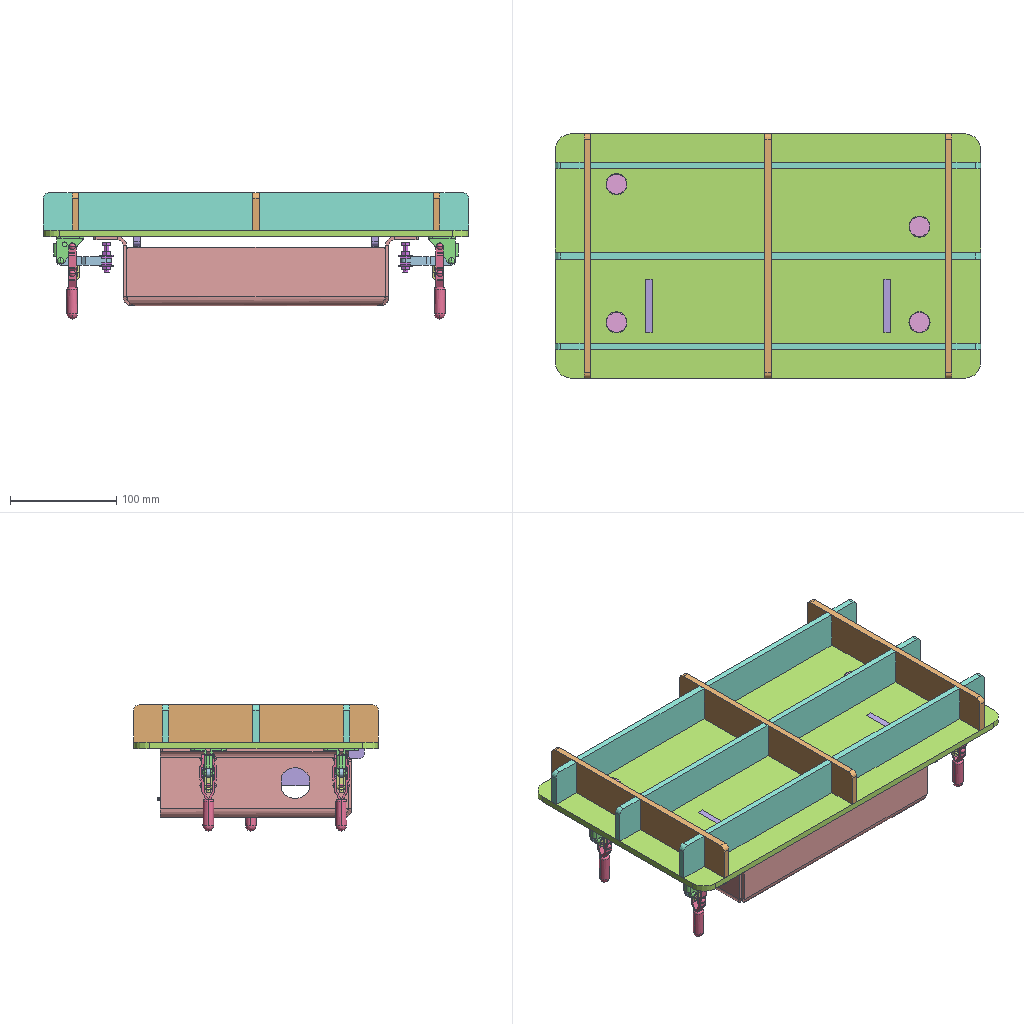Assembly | SolidWorks | 8 different items | 20 placed | box 400 x 230 x 119 mm
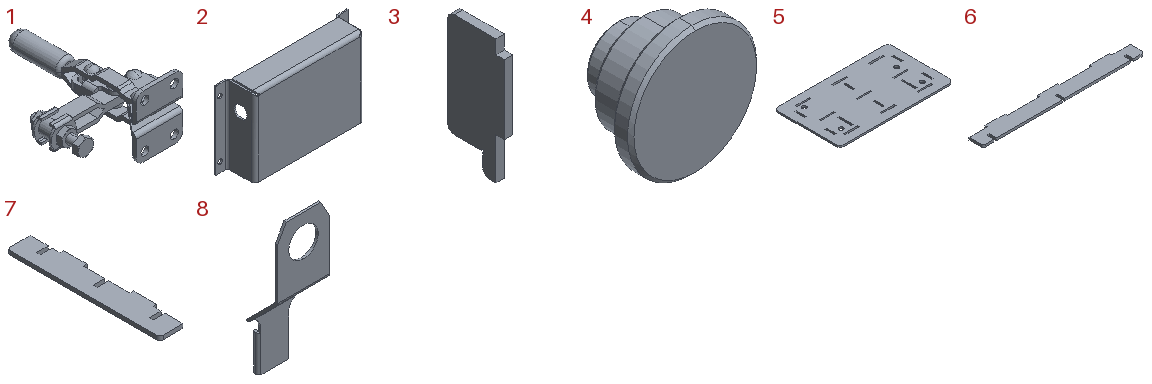Parts list (item | quantity | size | volume | features):
1 | x4 | 56.45 x 77.62 x 33.3 mm | 10418 mm3 | features BaseBody 5
2 | x1 | 305 x 65 x 180.2 mm | 266620 mm3 | features ICE 3, EdgeFlange 2, Fillet 1, FlatPattern 1, Fold 1, SMBaseFlange 1, SheetMetal 1, UnFold 1
3 | x2 | 6 x 41 x 90 mm | 18294 mm3 | features FlatPattern 1, SMBaseFlange 1, SheetMetal 1
4 | x4 | 20 x 12.2 x 20 mm | 2180 mm3 | features Chamfer 1, Revolution 1
5 | x1 | 400 x 230 x 6 mm | 519240 mm3 | features FlatPattern 1, SMBaseFlange 1, SheetMetal 1
6 | x3 | 400 x 40.5 x 6 mm | 86942 mm3 | features FlatPattern 1, SMBaseFlange 1, SheetMetal 1
7 | x3 | 40.5 x 230 x 6 mm | 48656 mm3 | features FlatPattern 1, SMBaseFlange 1, SheetMetal 1
8 | x2 | 23.06 x 15.573 x 65.7 mm | 1342 mm3 | features BaseBody 1
Mates (type | each side: item.copy, entity, surface, feature):
Coincident | 2.1 face plane Base-Flange1 | 8.1 face plane PN_0001.stp-1-solid1
DistanceDim | 8.1 face cylinder PN_0001.stp-1-solid1 | 2.1 face plane Base-Flange1
DistanceDim | 2.1 face plane Edge-Flange1 | 8.1 face cylinder PN_0001.stp-1-solid1
Parallel | 2.1 face plane Edge-Flange1 | 8.1 face plane PN_0001.stp-1-solid1
InPlace | 2.1 face plane Edge-Flange2 | 5.1 plane
InPlace | 4.1 plane | assembly plane
Concentric | 5.1 face cylinder Base-Flange1 | 4.2 face cylinder Revolve1
Coincident | 2.1 face plane Edge-Flange2 | 4.2 face plane Revolve1
Concentric | 2.1 face cylinder Cut-Extrude2 | 4.3 face cylinder Revolve1
Coincident | 2.1 face plane Edge-Flange2 | 4.3 face plane Revolve1
Concentric | 2.1 face cylinder Cut-Extrude2 | 4.4 face cylinder Revolve1
Coincident | 2.1 face plane Edge-Flange2 | 4.4 face plane Revolve1
InPlace | 6.1 plane | assembly plane
InPlace | 7.1 plane | assembly plane
Coincident | 5.1 face plane Base-Flange1 | 3.1 face plane Base-Flange1
Coincident | 2.1 face plane Edge-Flange1 | 3.1 face plane Base-Flange1
DistanceDim | 2.1 face plane Edge-Flange1 | 3.1 face plane Base-Flange1
Coincident | 5.1 face plane Base-Flange1 | 1.1 face plane TC1-1 Vertical flange base toggle clamp [TCS1-1].step-1/_TCS1-1(seat).step-1-solid1
DistanceDim | 1.1 face plane TC1-1 Vertical flange base toggle clamp [TCS1-1].step-1/_TCS1-1(bolt).step-1-solid1 | 2.1 face plane Edge-Flange2
DistanceDim | 2.1 face plane Edge-Flange2 | 1.1 face plane TC1-1 Vertical flange base toggle clamp [TCS1-1].step-1/_TCS1-1(seat).step-1-solid1
Coincident | 5.1 face plane Base-Flange1 | 1.2 face plane TC1-1 Vertical flange base toggle clamp [TCS1-1].step-1/_TCS1-1(seat).step-1-solid1
DistanceDim | 1.2 face plane TC1-1 Vertical flange base toggle clamp [TCS1-1].step-1/_TCS1-1(bolt).step-1-solid1 | 2.1 face plane Edge-Flange2
DistanceDim | 1.2 face plane TC1-1 Vertical flange base toggle clamp [TCS1-1].step-1/_TCS1-1(seat).step-1-solid1 | 2.1 face plane Edge-Flange2